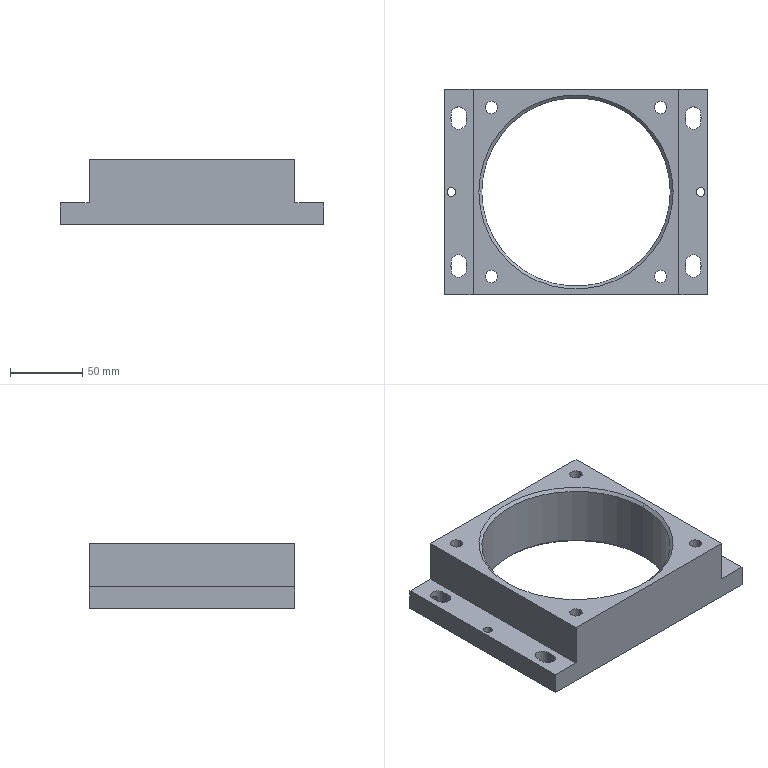Part | 1 solid | 68 faces | box 182 x 142 x 45 mm | volume 373309 mm3 | cylinder 38 | plane 26 | cone 4 | commonest cylinder face diameters 10.6 x12 8.5 x8 10.5 x8 6 x4 6.8 x4 130 x2